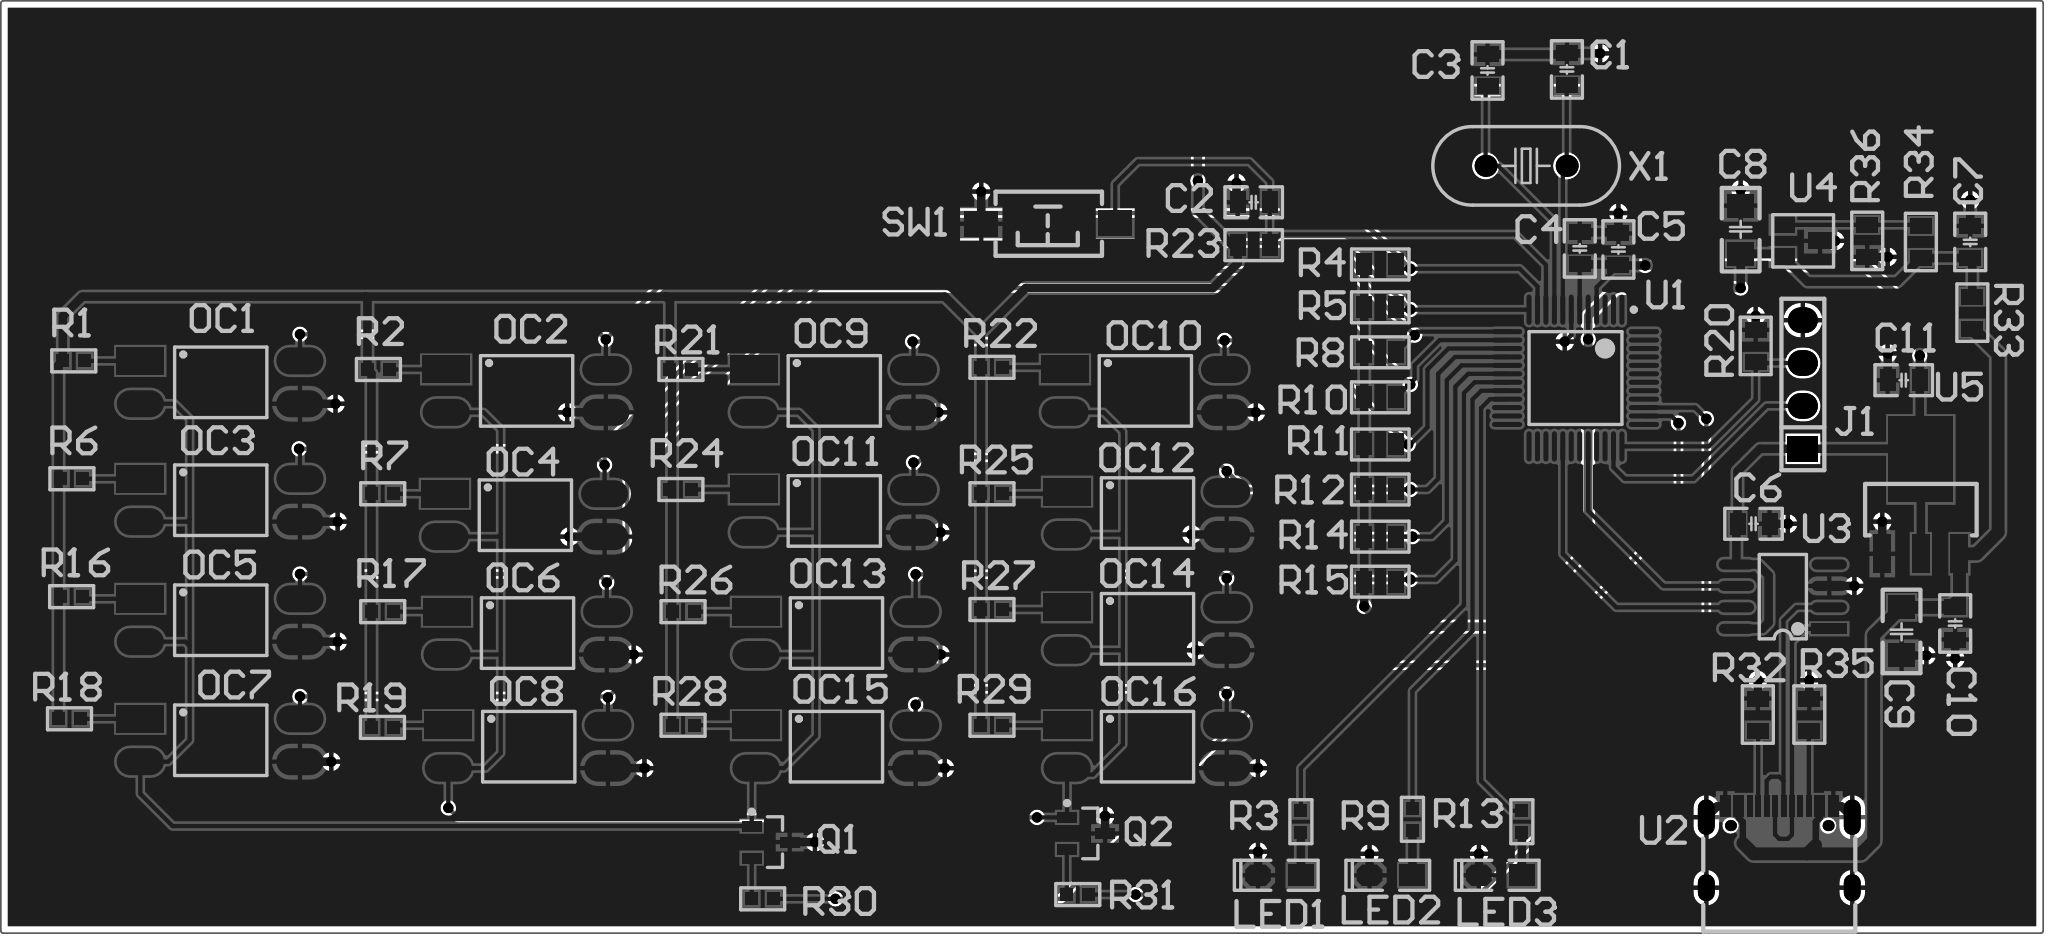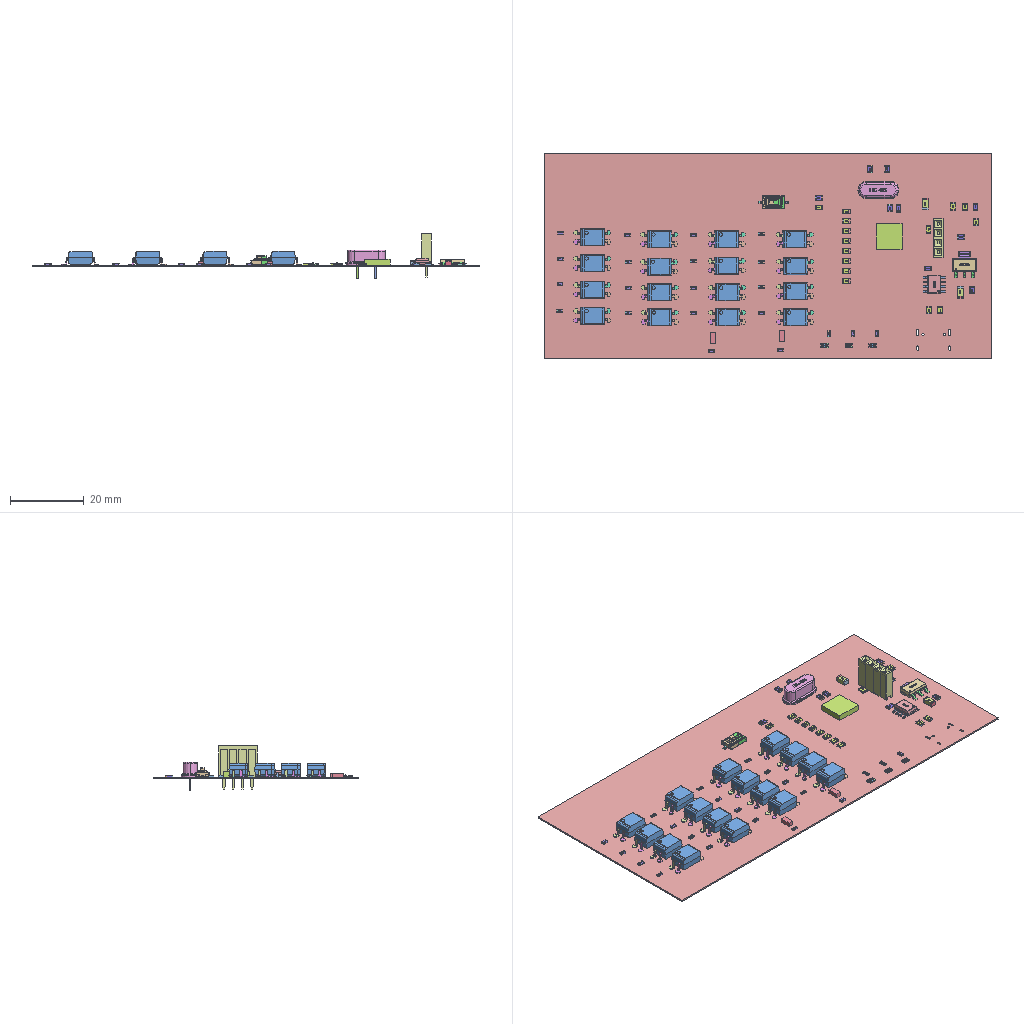Circuit board layout | Altium Designer | box 120.9 x 55.2 x 12 mm
Layer stack:
# Altium Designer layer stack of  (unit mm; dielectric type: 0 none, 1 core, 2 prepreg, 3 surface material)
index,name,kind,layer,copper_thickness_mm,dielectric_type,dielectric_thickness_mm,dielectric_material,dielectric_constant
0,Top Paste,other,,,,,,
1,Top Overlay,other,,,,,,
2,Top Solder,dielectric,,,3,0.0102,Solder Resist,3.5
3,Top Layer,copper,Top Layer,0.0356,,,,
4,Dielectric 1,dielectric,,,0,0.32,FR-4,4.8
5,Bottom Layer,copper,Bottom Layer,0.0356,,,,
6,Bottom Solder,dielectric,,,3,0.0102,Solder Resist,3.5
7,Bottom Overlay,other,,,,,,
8,Bottom Paste,other,,,,,,
# drill layer pairs: low layer,high layer
drill_pair,Top Layer,Bottom Layer
Part placement:
Designator,Comment,Layer,Footprint,Center-X(mm),Center-Y(mm),Rotation
X1,12MHz,TopLayer,OSC_HC-49S,121.92,108.458,360
U5,AMS1117,TopLayer,SOT223,145.288,88.265,360
U4,TL431DBZ,TopLayer,SOT-23,138.219,104.013,270
U3,CH340N,TopLayer,SOP8,137.116,82.931,180
U2,HC-TYPE-C-16P-01A COPY,TopLayer,USB-C-SMD_HC-TYPE-C-16P-01A,136.906,68.094,0
U1,STM32G030C8T6,TopLayer,LQFP48_N,124.841,95.885,270
SW1,3x6x5,TopLayer,TSW_SMD-3*6*2.5,93.628,105.039,180
R36,10K,TopLayer,R_0805_L,142.113,104.013,90
R35,5.1K,TopLayer,R_0805_L,138.684,75.946,270
R34,3.3K,TopLayer,R_0805_L,145.288,103.947,270
R33,330,TopLayer,R_0805_L,148.336,99.761,270
R32,5.1K,TopLayer,R_0805_L,135.636,75.946,270
R31,330,TopLayer,R_0603_L,95.377,65.278,180
R30,330,TopLayer,R_0603_L,76.723,65.024,180
R29,330,TopLayer,R_0603_L,90.297,75.311,360
R28,330,TopLayer,R_0603_L,72.009,75.311,360
R27,330,TopLayer,R_0603_L,90.297,82.169,360
R26,330,TopLayer,R_0603_L,72.009,82.042,360
R25,330,TopLayer,R_0603_L,90.297,89.027,360
R24,330,TopLayer,R_0603_L,71.882,89.281,360
R23,10K,TopLayer,R_0805_L,105.791,103.759,180
R22,330,TopLayer,R_0603_L,90.297,96.52,360
R21,330,TopLayer,R_0603_L,71.882,96.393,360
R20,10K,TopLayer,R_0805_L,135.509,97.79,270
R19,330,TopLayer,R_0603_L,54.214,75.184,360
R18,330,TopLayer,R_0603_L,35.687,75.692,360
R17,330,TopLayer,R_0603_L,54.229,82.042,360
R16,330,TopLayer,R_0603_L,35.814,82.931,360
R15,10K,TopLayer,R_0805_L,113.284,83.82,180
R14,10K,TopLayer,R_0805_L,113.284,86.487,180
R13,330,TopLayer,R_0603_L,121.666,69.596,90
R12,10K,TopLayer,R_0805_L,113.284,89.281,180
R11,10K,TopLayer,R_0805_L,113.284,91.948,180
R10,10K,TopLayer,R_0805_L,113.284,94.742,180
R9,330,TopLayer,R_0603_L,115.189,69.738,90
R8,10K,TopLayer,R_0805_L,113.284,97.409,180
R7,330,TopLayer,R_0603_L,54.229,89.027,0
R6,330,TopLayer,R_0603_L,35.829,89.916,0
R5,10K,TopLayer,R_0805_L,113.284,100.076,180
R4,10K,TopLayer,R_0805_L,113.284,102.616,180
R3,330,TopLayer,R_0603_L,108.585,69.596,90
R2,330,TopLayer,R_0603_L,53.975,96.393,0
R1,330,TopLayer,R_0603_L,35.941,96.901,0
Q2,QNPN,TopLayer,SOT-23B_N,95.867,68.9,0
Q1,QNPN,TopLayer,SOT-23B_N,77.198,68.387,0
OC16,ITR20001,TopLayer,SMD_PC817,99.468,74.041,360
OC15,ITR20001,TopLayer,SMD_PC817,81.053,74.041,360
OC14,ITR20001,TopLayer,SMD_PC817,99.468,81.026,360
OC13,ITR20001,TopLayer,SMD_PC817,81.053,80.772,360
OC12,ITR20001,TopLayer,SMD_PC817,99.468,87.884,360
OC11,ITR20001,TopLayer,SMD_PC817,80.926,88.011,360
OC10,ITR20001,TopLayer,SMD_PC817,99.341,95.123,360
OC9,ITR20001,TopLayer,SMD_PC817,80.926,95.123,360
OC8,ITR20001,TopLayer,SMD_PC817,62.838,74.041,360
OC7,ITR20001,TopLayer,SMD_PC817,44.604,74.422,360
OC6,ITR20001,TopLayer,SMD_PC817,62.765,80.772,360
OC5,ITR20001,TopLayer,SMD_PC817,44.604,81.534,360
OC4,ITR20001,TopLayer,SMD_PC817,62.638,87.757,360
OC3,ITR20001,TopLayer,SMD_PC817,44.604,88.646,360
OC2,ITR20001,TopLayer,SMD_PC817,62.711,95.123,360
OC1,ITR20001,TopLayer,SMD_PC817,44.604,95.631,360
LED3,Red,TopLayer,LED_0805G,120.396,66.421,180
LED2,Red,TopLayer,LED_0805G,113.919,66.421,180
LED1,Red,TopLayer,LED_0805G,107.315,66.421,180
J1,Female HDR1X4,TopLayer,Fe-HDR1X4/2.54-S,138.303,95.504,180
C11,0.1UF,TopLayer,C_0805_L,144.272,95.758,0
C10,0.1UF,TopLayer,C_0805_L,147.32,81.341,90
C9,30UF,TopLayer,C_1206_L,144.145,80.871,90
C8,10UF,TopLayer,C_1206_L,134.62,104.676,270
C7,0.1UF,TopLayer,C_0805_L,148.209,103.952,270
C6,0.1UF,TopLayer,C_0805_L,135.382,87.249,180
C5,0.1UF,TopLayer,C_0805_L,127.381,103.505,270
C4,0.1UF,TopLayer,C_0805_L,125.095,103.566,270
C3,22PF,TopLayer,C_0805_L,119.634,114.112,90
C2,0.1UF,TopLayer,C_0805_L,105.791,106.299,0
C1,22PF,TopLayer,C_0805_L,124.333,114.173,270
Pad and via stacks:
# Altium Designer via and pad stacks of  (unit mm). Each distinct definition once, with the count of objects using it.
# via: kind,start_layer,end_layer,hole_mm,diameter_mm,mode(0 simple;1 top-mid-bottom;2 full stack),diameter_per_layer,count,example_net
# pad: kind,layer,hole_mm,hole_type(0 round;1 square;2 slot),plating,top_size,top_shape(1 round;2 rect;3 octagon;9 rounded rect),mid_size,bottom_size,mode,footprint,size_per_layer,count,example
pad,Top Layer,0,0,plated,1.6x2.8,1,1.6x2.8,1.6x2.8,0,SMD_PC817,,48,OC2.3
pad,Top Layer,0,0,plated,1.6x2.8,2,1.6x2.8,1.6x2.8,0,SMD_PC817,,16,OC2.1
pad,Top Layer,0,0,plated,0.762x0.762,2,0.762x0.762,0.762x0.762,0,R 0603_L,,42,R2.2
pad,Top Layer,0,0,plated,0.3x1.8,1,0.3x1.8,0.3x1.8,0,LQFP48_N,,48,U1.48
pad,Top Layer,0,0,plated,1.27x0.889,2,1.27x0.889,1.27x0.889,0,R 0805_L,,30,R4.1
pad,Top Layer,0,0,plated,1.524x1.27,2,1.524x1.27,1.524x1.27,0,LED 0805G,,3,LED1.1
pad,Top Layer,0,0,plated,1.524x1.27,3,1.524x1.27,1.524x1.27,0,LED 0805G,,3,LED1.2
pad,Top Layer,0,0,plated,2x1.5,2,2x1.5,2x1.5,0,TSW SMD-3*6*2.5,,2,SW1.1
pad,Top Layer,0,0,plated,1.27x0.889,2,1.27x0.889,1.27x0.889,0,C 0805_L,,18,C1.1
pad,Top Layer,0,0,plated,0.6x1.15,2,0.6x1.15,0.6x1.15,0,SOT-23B_N,,6,Q2.1
pad,Top Layer,0,0,plated,0.6x1.3,2,0.6x1.3,0.6x1.3,0,USB-C-SMD_HC-TYPE-C-16P-01A,,4,U2.B1A12
pad,Top Layer,0,0,plated,0.3x1.3,2,0.3x1.3,0.3x1.3,0,USB-C-SMD_HC-TYPE-C-16P-01A,,8,U2.B5
pad,Top Layer,0,0,plated,0.6x2.1,1,0.6x2.1,0.6x2.1,0,SOP8,,7,U3.5
pad,Top Layer,0,0,plated,0.6x2.1,2,0.6x2.1,0.6x2.1,0,SOP8,,1,U3.1
pad,Top Layer,0,0,plated,1.397x1.575,2,1.397x1.575,1.397x1.575,0,C 1206_L,,4,C8.2
pad,Top Layer,0,0,plated,1.016x2.286,2,1.016x2.286,1.016x2.286,0,SOT223,,3,U5.3
pad,Top Layer,0,0,plated,3.81x5.08,2,3.81x5.08,3.81x5.08,0,SOT223,,1,U5.2
pad,Top Layer,0,0,plated,1x1.4,2,1x1.4,1x1.4,0,SOT-23,,3,U4.2
pad,Multi-Layer,0.8128,0,plated,1.524x1.778,1,1.524x1.778,1.524x1.778,0,Fe-HDR1X4/2.54-S,,3,J1.4
pad,Multi-Layer,0.8128,0,plated,1.524x1.778,2,1.524x1.778,1.524x1.778,0,Fe-HDR1X4/2.54-S,,1,J1.1
pad,Multi-Layer,0.6,0,plated,1.3x1.3,1,1.3x1.3,1.3x1.3,0,OSC HC-49S,,2,X1.2
pad,Multi-Layer,0.6,2,plated,1x2.1,1,1x2.1,1x2.1,0,USB-C-SMD_HC-TYPE-C-16P-01A,,2,U2.1
pad,Multi-Layer,0.6,2,plated,1x1.6,1,1x1.6,1x1.6,0,USB-C-SMD_HC-TYPE-C-16P-01A,,2,U2.4
pad,Multi-Layer,0.65,0,unplated,0.65x0.65,1,0.65x0.65,0.65x0.65,0,USB-C-SMD_HC-TYPE-C-16P-01A,,2,U2.
via,Top Layer,Bottom Layer,0.3048,0.6096,0,,75,GND
Copper pours:
name,layer,net,type(0 solid;1 hatched;2 none)
D,Top Layer,GND,0
D,Bottom Layer,GND,0
Design rules, without the lines most boards share:
# Altium Designer design rules of  (exported by Altium Designer, unit mm)
# columns: name | kind | enabled | priority | scope1 | scope2 | descriptor | typed fields (field=value)
Clearance | 0 | enabled | 1 | All | All | Clearance Constraint (Gap=6mil) (All),(All) | gap=0.1524
PlaneConnect | 6 | enabled | 1 | All | All | Power Plane Connect Rule(Relief Connect )(Expansion=20mil) (Conductor Width=10mil) (Air Gap=10mil) (Entries=4) (All) | relief_conductor_width=0.254 relief_entries=4 relief_expansion=0.508
PolygonConnect | 20 | enabled | 1 | All | All | Polygon Connect Rule(Relief Connect )(Conductor Width=10mil) (Relief Angle=90 Angle) (Entries=4) (Air Gap Width=10mil) (All),(All) | connect_style(0=relief,1=direct,2=none)=0 relief_conductor_width=0.254 relief_entries=4
Width | 2 | enabled | 1 | All | All | Width Constraint (Min=10mil) (Max=50mil) (Preferred=10mil) (All) |
RoutingVias | 11 | enabled | 1 | All | All | Routing Via (MinHoleWidth=28mil) (MaxHoleWidth=28mil) (PreferredHoleWidth=28mil) (MinWidth=50mil) (MaxWidth=50mil) (PreferedWidth=50mil) (All) | via_min_hole=0.7112 via_max_hole=0.7112 via_preferred_diameter=1.27 via_preferred_hole=0.7112
PasteMaskExpansion | 14 | enabled | 1 | All | All | Paste Mask Expansion (Expansion =0mil) (All) | expansion=0
SolderMaskExpansion | 13 | enabled | 1 | All | All | Solder Mask Expansion (Expansion =4mil) (All) | expansion=0.1016
DiffPairsRouting | 51 | enabled | 1 | All | All | Differential Pairs Uncoupled Length using the Gap Constraints (Min=10mil) (Max=10mil) (Prefered=10mil)  and Width Constraints (Min=15mil) (Max=15mil) (Prefered=15mil) (All) |
HoleToHoleClearance | 52 | enabled | 1 | All | All | Hole To Hole Clearance (Gap=10mil) (All),(All) | gap=0.254
MinimumSolderMaskSliver | 53 | enabled | 1 | All | All | Minimum Solder Mask Sliver (Gap=0mil) (All),(All) |
SilkToSolderMaskClearance | 54 | enabled | 1 | IsPad | All | Silk To Solder Mask (Clearance=0mil) (IsPad),(All) |
SilkToSilkClearance | 55 | enabled | 1 | All | All | Silk to Silk (Clearance=0mil) (All),(All) |
Classes set for this board:
# Altium Designer classes of  (member kind: 0 net, 1 component, 2 from-to, 3 pad, 4 layer, 5 differential pair, 6 design channel, 7 polygon, 8 structure, 9 xSignal)
# columns: class name | member kind | superclass | members
Sheet1 | 1 | no | C1; C2; C3; C4; C5; C6; C7; C8; C9; C10; C11; J1; LED1; LED2; LED3; OC1; OC2; OC3; OC4; OC5; OC6; OC7; OC8; OC9; OC10; OC11; OC12; OC13; OC14; OC15; OC16; Q1; Q2; R1; R2; R3; R4; R5; R6; R7; R8; R9; R10; R11; R12; R13; R14; R15; R16; R17; R18; R19; R20; R21; R22; R23; R24; R25; R26; R27; R28; R29; R30; R31; R32; R33; R34; R35; R36; SW1; U1; U2; U3; U4; U5; X1;